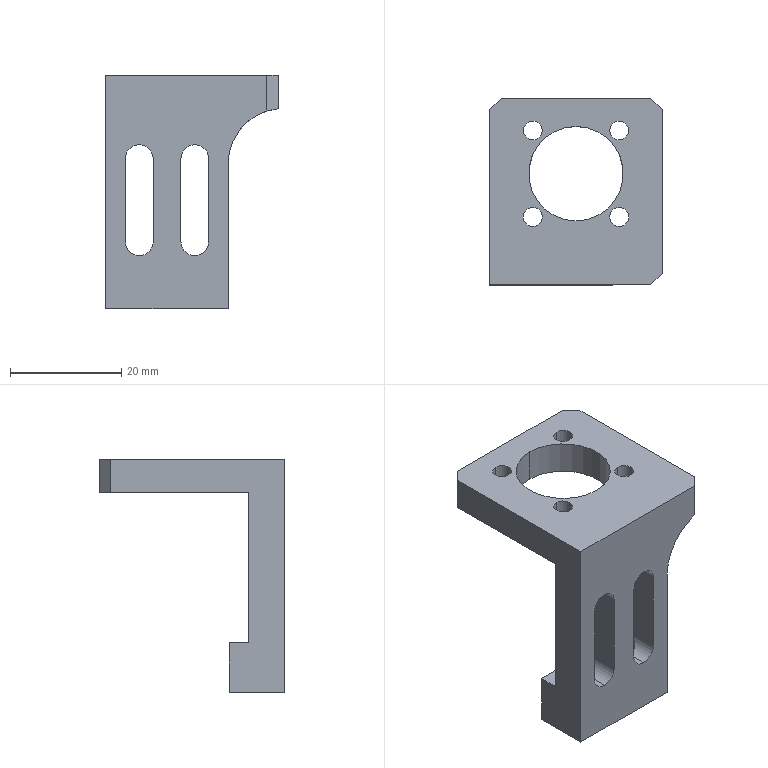NC program | NX | posted with a generic post | part box 31 x 33.478 x 42 mm
Lines 1 to 47 of 3423:
N10 G17 G21 G94 G90
(FLOOR_WALL , TOOL : D80)
N12 T19 M6
N14 G54
N16 G17 G0 G90 X-60.5 Y0. B0. C0. S6500 M3
N18 G43 Z30. H19
N20 Z3.
N22 G94 G1 Z0. F1500.
N24 X-57.5
N26 X57.5
N28 X60.5
N30 Z3.
N32 G0 Z30.
N34 M5
(DRILLING , TOOL : D6A45)
N36 T01 M6
N38 G54
N40 G17 G0 G90 X-7.778 Y11.039 B0. C0. S9500 M3
N42 G43 Z30. H1
N44 G94 G81 G98 Z-1. F250. R3.
N46 X7.778
N48 X0. Y3.261
N50 X-7.778 Y-4.517
N52 X7.778
N54 G80
N56 G0 X7.778 Y-4.517 Z30.
N58 M5
(DRILLING_COPY_COPY_COPY , TOOL : 3.4ZT)
N60 T16 M6
N62 G54
N64 G17 G0 G90 X7.778 Y11.039 B0. C0. S2000 M3
N66 G43 Z30. H16
N68 G94 G83 G98 Z-8.521 F200. Q2. R3.
N70 X-7.778
N72 Y-4.517
N74 X7.778
N76 G80
N78 G0 X7.778 Y-4.517 Z30.
N80 M5